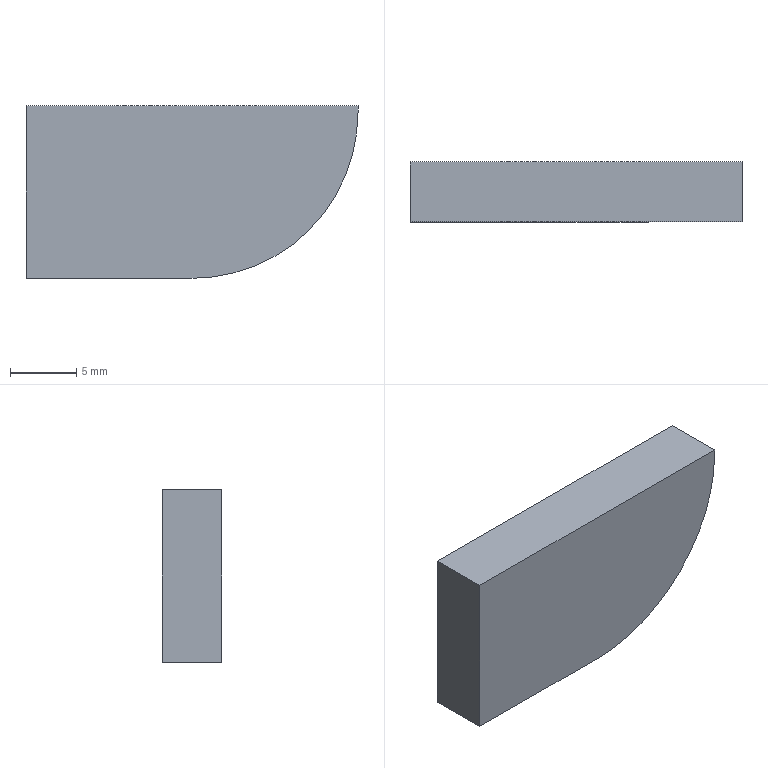Part | SolidWorks | features Extrusion 1 | 1 solid | 7 faces | box 25 x 4.5 x 13 mm | volume 1312 mm3 | plane 6 | cylinder 1 | commonest cylinder face diameters 25 x1
STEP:
#1=CARTESIAN_POINT('',(0.,-2.25,-13.));
#2=VERTEX_POINT('',#1);
#3=CARTESIAN_POINT('',(0.,-2.25,0.));
#4=VERTEX_POINT('',#3);
#5=CARTESIAN_POINT('',(0.,-2.25,0.));
#6=DIRECTION('',(0.,0.,1.));
#7=VECTOR('',#6,1000.);
#8=LINE('',#5,#7);
#9=EDGE_CURVE('',#2,#4,#8,.T.);
#10=ORIENTED_EDGE('',*,*,#9,.T.);
#11=CARTESIAN_POINT('',(0.,2.25,0.));
#12=VERTEX_POINT('',#11);
#13=CARTESIAN_POINT('',(0.,2.25,0.));
#14=DIRECTION('',(0.,-1.,0.));
#15=VECTOR('',#14,1000.);
#16=LINE('',#13,#15);
#17=EDGE_CURVE('',#12,#4,#16,.T.);
#18=ORIENTED_EDGE('',*,*,#17,.F.);
#19=CARTESIAN_POINT('',(0.,2.25,-13.));
#20=VERTEX_POINT('',#19);
#21=CARTESIAN_POINT('',(0.,2.25,0.));
#22=DIRECTION('',(0.,0.,1.));
#23=VECTOR('',#22,1000.);
#24=LINE('',#21,#23);
#25=EDGE_CURVE('',#20,#12,#24,.T.);
#26=ORIENTED_EDGE('',*,*,#25,.F.);
#27=CARTESIAN_POINT('',(0.,2.25,-13.));
#28=DIRECTION('',(0.,-1.,0.));
#29=VECTOR('',#28,1000.);
#30=LINE('',#27,#29);
#31=EDGE_CURVE('',#20,#2,#30,.T.);
#32=ORIENTED_EDGE('',*,*,#31,.T.);
#33=EDGE_LOOP('',(#10,#18,#26,#32));
#34=FACE_OUTER_BOUND('',#33,.T.);
#35=CARTESIAN_POINT('',(0.,2.25,0.));
#36=DIRECTION('',(1.,0.,0.));
#37=DIRECTION('',(0.,0.,-1.));
#38=AXIS2_PLACEMENT_3D('',#35,#36,#37);
#39=PLANE('',#38);
#40=ADVANCED_FACE('',(#34),#39,.F.);
#41=CARTESIAN_POINT('',(25.,-2.25,0.));
#42=VERTEX_POINT('',#41);
#43=CARTESIAN_POINT('',(0.,-2.25,0.));
#44=DIRECTION('',(1.,0.,0.));
#45=VECTOR('',#44,1000.);
#46=LINE('',#43,#45);
#47=EDGE_CURVE('',#4,#42,#46,.T.);
#48=ORIENTED_EDGE('',*,*,#47,.T.);
#49=CARTESIAN_POINT('',(25.,2.25,0.));
#50=VERTEX_POINT('',#49);
#51=CARTESIAN_POINT('',(25.,2.25,0.));
#52=DIRECTION('',(0.,-1.,0.));
#53=VECTOR('',#52,1000.);
#54=LINE('',#51,#53);
#55=EDGE_CURVE('',#50,#42,#54,.T.);
#56=ORIENTED_EDGE('',*,*,#55,.F.);
#57=CARTESIAN_POINT('',(0.,2.25,0.));
#58=DIRECTION('',(1.,0.,0.));
#59=VECTOR('',#58,1000.);
#60=LINE('',#57,#59);
#61=EDGE_CURVE('',#12,#50,#60,.T.);
#62=ORIENTED_EDGE('',*,*,#61,.F.);
#63=ORIENTED_EDGE('',*,*,#17,.T.);
#64=EDGE_LOOP('',(#48,#56,#62,#63));
#65=FACE_OUTER_BOUND('',#64,.T.);
#66=CARTESIAN_POINT('',(0.,2.25,0.));
#67=DIRECTION('',(0.,0.,-1.));
#68=DIRECTION('',(-1.,0.,0.));
#69=AXIS2_PLACEMENT_3D('',#66,#67,#68);
#70=PLANE('',#69);
#71=ADVANCED_FACE('',(#65),#70,.F.);
#72=CARTESIAN_POINT('',(25.,-2.25,-0.5));
#73=VERTEX_POINT('',#72);
#74=CARTESIAN_POINT('',(25.,-2.25,0.));
#75=DIRECTION('',(0.,0.,-1.));
#76=VECTOR('',#75,1000.);
#77=LINE('',#74,#76);
#78=EDGE_CURVE('',#42,#73,#77,.T.);
#79=ORIENTED_EDGE('',*,*,#78,.T.);
#80=CARTESIAN_POINT('',(25.,2.25,-0.5));
#81=VERTEX_POINT('',#80);
#82=CARTESIAN_POINT('',(25.,2.25,-0.5));
#83=DIRECTION('',(0.,-1.,0.));
#84=VECTOR('',#83,1000.);
#85=LINE('',#82,#84);
#86=EDGE_CURVE('',#81,#73,#85,.T.);
#87=ORIENTED_EDGE('',*,*,#86,.F.);
#88=CARTESIAN_POINT('',(25.,2.25,0.));
#89=DIRECTION('',(0.,0.,-1.));
#90=VECTOR('',#89,1000.);
#91=LINE('',#88,#90);
#92=EDGE_CURVE('',#50,#81,#91,.T.);
#93=ORIENTED_EDGE('',*,*,#92,.F.);
#94=ORIENTED_EDGE('',*,*,#55,.T.);
#95=EDGE_LOOP('',(#79,#87,#93,#94));
#96=FACE_OUTER_BOUND('',#95,.T.);
#97=CARTESIAN_POINT('',(25.,2.25,0.));
#98=DIRECTION('',(-1.,0.,0.));
#99=DIRECTION('',(0.,0.,1.));
#100=AXIS2_PLACEMENT_3D('',#97,#98,#99);
#101=PLANE('',#100);
#102=ADVANCED_FACE('',(#96),#101,.F.);
#103=CARTESIAN_POINT('',(12.5,-2.25,-13.));
#104=VERTEX_POINT('',#103);
#105=CARTESIAN_POINT('',(12.5,-2.25,-0.5));
#106=DIRECTION('',(0.,1.,0.));
#107=DIRECTION('',(0.,0.,-1.));
#108=AXIS2_PLACEMENT_3D('',#105,#106,#107);
#109=CIRCLE('',#108,12.5);
#110=EDGE_CURVE('',#73,#104,#109,.T.);
#111=ORIENTED_EDGE('',*,*,#110,.T.);
#112=CARTESIAN_POINT('',(12.5,2.25,-13.));
#113=VERTEX_POINT('',#112);
#114=CARTESIAN_POINT('',(12.5,2.25,-13.));
#115=DIRECTION('',(0.,-1.,0.));
#116=VECTOR('',#115,1000.);
#117=LINE('',#114,#116);
#118=EDGE_CURVE('',#113,#104,#117,.T.);
#119=ORIENTED_EDGE('',*,*,#118,.F.);
#120=CARTESIAN_POINT('',(12.5,2.25,-0.5));
#121=DIRECTION('',(0.,1.,0.));
#122=DIRECTION('',(0.,0.,-1.));
#123=AXIS2_PLACEMENT_3D('',#120,#121,#122);
#124=CIRCLE('',#123,12.5);
#125=EDGE_CURVE('',#81,#113,#124,.T.);
#126=ORIENTED_EDGE('',*,*,#125,.F.);
#127=ORIENTED_EDGE('',*,*,#86,.T.);
#128=EDGE_LOOP('',(#111,#119,#126,#127));
#129=FACE_OUTER_BOUND('',#128,.T.);
#130=CARTESIAN_POINT('',(12.5,2.25,-0.5));
#131=DIRECTION('',(0.,-1.,0.));
#132=DIRECTION('',(0.,0.,-1.));
#133=AXIS2_PLACEMENT_3D('',#130,#131,#132);
#134=CYLINDRICAL_SURFACE('',#133,12.5);
#135=ADVANCED_FACE('',(#129),#134,.T.);
#136=CARTESIAN_POINT('',(0.,-2.25,-13.));
#137=DIRECTION('',(-1.,0.,0.));
#138=VECTOR('',#137,1000.);
#139=LINE('',#136,#138);
#140=EDGE_CURVE('',#104,#2,#139,.T.);
#141=ORIENTED_EDGE('',*,*,#140,.T.);
#142=ORIENTED_EDGE('',*,*,#31,.F.);
#143=CARTESIAN_POINT('',(0.,2.25,-13.));
#144=DIRECTION('',(-1.,0.,0.));
#145=VECTOR('',#144,1000.);
#146=LINE('',#143,#145);
#147=EDGE_CURVE('',#113,#20,#146,.T.);
#148=ORIENTED_EDGE('',*,*,#147,.F.);
#149=ORIENTED_EDGE('',*,*,#118,.T.);
#150=EDGE_LOOP('',(#141,#142,#148,#149));
#151=FACE_OUTER_BOUND('',#150,.T.);
#152=CARTESIAN_POINT('',(0.,2.25,-13.));
#153=DIRECTION('',(0.,0.,1.));
#154=DIRECTION('',(1.,0.,0.));
#155=AXIS2_PLACEMENT_3D('',#152,#153,#154);
#156=PLANE('',#155);
#157=ADVANCED_FACE('',(#151),#156,.F.);
#158=ORIENTED_EDGE('',*,*,#25,.T.);
#159=ORIENTED_EDGE('',*,*,#61,.T.);
#160=ORIENTED_EDGE('',*,*,#92,.T.);
#161=ORIENTED_EDGE('',*,*,#125,.T.);
#162=ORIENTED_EDGE('',*,*,#147,.T.);
#163=EDGE_LOOP('',(#158,#159,#160,#161,#162));
#164=FACE_OUTER_BOUND('',#163,.T.);
#165=CARTESIAN_POINT('',(12.5,2.25,-0.5));
#166=DIRECTION('',(0.,-1.,0.));
#167=DIRECTION('',(0.,0.,-1.));
#168=AXIS2_PLACEMENT_3D('',#165,#166,#167);
#169=PLANE('',#168);
#170=ADVANCED_FACE('',(#164),#169,.F.);
#171=ORIENTED_EDGE('',*,*,#9,.F.);
#172=ORIENTED_EDGE('',*,*,#140,.F.);
#173=ORIENTED_EDGE('',*,*,#110,.F.);
#174=ORIENTED_EDGE('',*,*,#78,.F.);
#175=ORIENTED_EDGE('',*,*,#47,.F.);
#176=EDGE_LOOP('',(#171,#172,#173,#174,#175));
#177=FACE_OUTER_BOUND('',#176,.T.);
#178=CARTESIAN_POINT('',(12.5,-2.25,-0.5));
#179=DIRECTION('',(0.,-1.,0.));
#180=DIRECTION('',(0.,0.,-1.));
#181=AXIS2_PLACEMENT_3D('',#178,#179,#180);
#182=PLANE('',#181);
#183=ADVANCED_FACE('',(#177),#182,.T.);
#184=CLOSED_SHELL('',(#40,#71,#102,#135,#157,#170,#183));
#185=MANIFOLD_SOLID_BREP('',#184);
#186=CARTESIAN_POINT('',(0.,0.,0.));
#187=DIRECTION('',(0.,0.,1.));
#188=DIRECTION('',(1.,0.,0.));
#189=AXIS2_PLACEMENT_3D('',#186,#187,#188);
#190=(LENGTH_UNIT()NAMED_UNIT(*)SI_UNIT(.MILLI.,.METRE.));
#191=UNCERTAINTY_MEASURE_WITH_UNIT(LENGTH_MEASURE(0.00001),#190,'','');
#192=(NAMED_UNIT(*)PLANE_ANGLE_UNIT()SI_UNIT($,.RADIAN.));
#193=(NAMED_UNIT(*)SI_UNIT($,.STERADIAN.)SOLID_ANGLE_UNIT());
#194=(GEOMETRIC_REPRESENTATION_CONTEXT(3)GLOBAL_UNCERTAINTY_ASSIGNED_CONTEXT((#191))GLOBAL_UNIT_ASSIGNED_CONTEXT((#190,#192,#193))REPRESENTATION_CONTEXT('',''));
#195=ADVANCED_BREP_SHAPE_REPRESENTATION('',(#185,#189),#194);